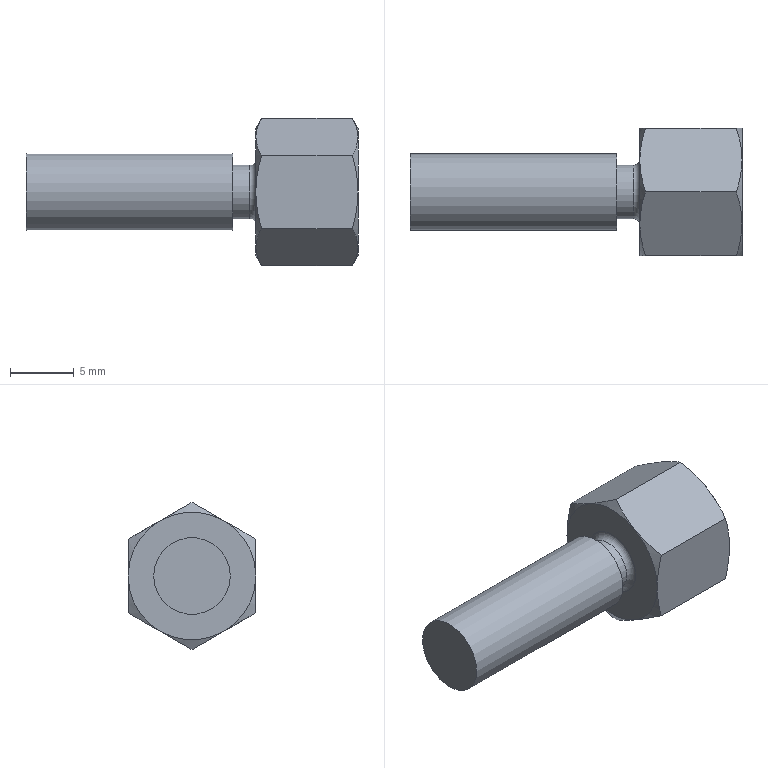Part | NX | features 5003_319_JPRAM6-L8.00-F18 2 | 1 solid | 25 faces | box 26 x 10 x 11.547 mm | volume 1174 mm3 | cone 12 | plane 10 | cylinder 2 | torus 1 | commonest cylinder face diameters 4.2 x1 6 x1
STEP:
#1=CARTESIAN_POINT('',(36.078,-172.,-214.226));
#2=VERTEX_POINT('',#1);
#3=CARTESIAN_POINT('',(28.972,-172.,-214.226));
#4=VERTEX_POINT('',#3);
#5=CARTESIAN_POINT('',(36.525,-172.,-214.226));
#6=DIRECTION('',(-1.,0.,0.));
#7=VECTOR('',#6,1000.);
#8=LINE('',#5,#7);
#9=EDGE_CURVE('',#2,#4,#8,.T.);
#10=ORIENTED_EDGE('',*,*,#9,.F.);
#11=CARTESIAN_POINT('',(36.525,-169.5,-215.67));
#12=VERTEX_POINT('',#11);
#13=CARTESIAN_POINT('',(36.078,-172.,-214.226));
#14=CARTESIAN_POINT('',(36.351,-171.182,-214.699));
#15=CARTESIAN_POINT('',(36.525,-170.352,-215.178));
#16=CARTESIAN_POINT('',(36.525,-169.5,-215.67));
#17=B_SPLINE_CURVE_WITH_KNOTS('',3,(#13,#14,#15,#16),.UNSPECIFIED.,.F.,.F.,(4,4),(0.000000238,0.002921),.UNSPECIFIED.);
#18=EDGE_CURVE('',#2,#12,#17,.T.);
#19=ORIENTED_EDGE('',*,*,#18,.T.);
#20=CARTESIAN_POINT('',(36.078,-167.,-217.113));
#21=VERTEX_POINT('',#20);
#22=CARTESIAN_POINT('',(36.525,-169.5,-215.67));
#23=CARTESIAN_POINT('',(36.525,-168.651,-216.16));
#24=CARTESIAN_POINT('',(36.35,-167.816,-216.642));
#25=CARTESIAN_POINT('',(36.078,-167.,-217.113));
#26=B_SPLINE_CURVE_WITH_KNOTS('',3,(#22,#23,#24,#25),.UNSPECIFIED.,.F.,.F.,(4,4),(0.002921,0.005831),.UNSPECIFIED.);
#27=EDGE_CURVE('',#12,#21,#26,.T.);
#28=ORIENTED_EDGE('',*,*,#27,.T.);
#29=CARTESIAN_POINT('',(28.972,-167.,-217.113));
#30=VERTEX_POINT('',#29);
#31=CARTESIAN_POINT('',(36.525,-167.,-217.113));
#32=DIRECTION('',(-1.,0.,0.));
#33=VECTOR('',#32,1000.);
#34=LINE('',#31,#33);
#35=EDGE_CURVE('',#21,#30,#34,.T.);
#36=ORIENTED_EDGE('',*,*,#35,.T.);
#37=CARTESIAN_POINT('',(28.525,-169.5,-215.67));
#38=VERTEX_POINT('',#37);
#39=CARTESIAN_POINT('',(28.972,-167.,-217.113));
#40=CARTESIAN_POINT('',(28.699,-167.818,-216.641));
#41=CARTESIAN_POINT('',(28.525,-168.648,-216.162));
#42=CARTESIAN_POINT('',(28.525,-169.5,-215.67));
#43=B_SPLINE_CURVE_WITH_KNOTS('',3,(#39,#40,#41,#42),.UNSPECIFIED.,.F.,.F.,(4,4),(0.000000238,0.002921),.UNSPECIFIED.);
#44=EDGE_CURVE('',#30,#38,#43,.T.);
#45=ORIENTED_EDGE('',*,*,#44,.T.);
#46=CARTESIAN_POINT('',(28.525,-169.5,-215.67));
#47=CARTESIAN_POINT('',(28.525,-170.349,-215.18));
#48=CARTESIAN_POINT('',(28.7,-171.184,-214.698));
#49=CARTESIAN_POINT('',(28.972,-172.,-214.226));
#50=B_SPLINE_CURVE_WITH_KNOTS('',3,(#46,#47,#48,#49),.UNSPECIFIED.,.F.,.F.,(4,4),(0.002921,0.005831),.UNSPECIFIED.);
#51=EDGE_CURVE('',#38,#4,#50,.T.);
#52=ORIENTED_EDGE('',*,*,#51,.T.);
#53=EDGE_LOOP('',(#10,#19,#28,#36,#45,#52));
#54=FACE_BOUND('',#53,.T.);
#55=CARTESIAN_POINT('',(36.525,-172.,-214.226));
#56=DIRECTION('',(0.,0.5,0.866));
#57=DIRECTION('',(0.,-0.866,0.5));
#58=AXIS2_PLACEMENT_3D('',#55,#56,#57);
#59=PLANE('',#58);
#60=ADVANCED_FACE('',(#54),#59,.T.);
#61=ORIENTED_EDGE('',*,*,#35,.F.);
#62=CARTESIAN_POINT('',(36.525,-167.,-220.));
#63=VERTEX_POINT('',#62);
#64=CARTESIAN_POINT('',(36.525,-167.,-220.));
#65=CARTESIAN_POINT('',(36.525,-167.,-219.024));
#66=CARTESIAN_POINT('',(36.348,-167.,-218.047));
#67=CARTESIAN_POINT('',(36.078,-167.,-217.113));
#68=B_SPLINE_CURVE_WITH_KNOTS('',3,(#64,#65,#66,#67),.UNSPECIFIED.,.F.,.F.,(4,4),(0.008071,0.01099),.UNSPECIFIED.);
#69=EDGE_CURVE('',#21,#63,#68,.F.);
#70=ORIENTED_EDGE('',*,*,#69,.T.);
#71=CARTESIAN_POINT('',(36.078,-167.,-222.887));
#72=VERTEX_POINT('',#71);
#73=CARTESIAN_POINT('',(36.078,-167.,-222.887));
#74=CARTESIAN_POINT('',(36.349,-167.,-221.948));
#75=CARTESIAN_POINT('',(36.525,-167.,-220.976));
#76=CARTESIAN_POINT('',(36.525,-167.,-220.));
#77=B_SPLINE_CURVE_WITH_KNOTS('',3,(#73,#74,#75,#76),.UNSPECIFIED.,.F.,.F.,(4,4),(0.00515,0.008071),.UNSPECIFIED.);
#78=EDGE_CURVE('',#63,#72,#77,.F.);
#79=ORIENTED_EDGE('',*,*,#78,.T.);
#80=CARTESIAN_POINT('',(28.972,-167.,-222.887));
#81=VERTEX_POINT('',#80);
#82=CARTESIAN_POINT('',(36.525,-167.,-222.887));
#83=DIRECTION('',(-1.,0.,0.));
#84=VECTOR('',#83,1000.);
#85=LINE('',#82,#84);
#86=EDGE_CURVE('',#72,#81,#85,.T.);
#87=ORIENTED_EDGE('',*,*,#86,.T.);
#88=CARTESIAN_POINT('',(28.525,-167.,-220.));
#89=VERTEX_POINT('',#88);
#90=CARTESIAN_POINT('',(28.972,-167.,-222.887));
#91=CARTESIAN_POINT('',(28.701,-167.,-221.948));
#92=CARTESIAN_POINT('',(28.525,-167.,-220.976));
#93=CARTESIAN_POINT('',(28.525,-167.,-220.));
#94=B_SPLINE_CURVE_WITH_KNOTS('',3,(#90,#91,#92,#93),.UNSPECIFIED.,.F.,.F.,(4,4),(0.00515,0.008071),.UNSPECIFIED.);
#95=EDGE_CURVE('',#81,#89,#94,.T.);
#96=ORIENTED_EDGE('',*,*,#95,.T.);
#97=CARTESIAN_POINT('',(28.525,-167.,-220.));
#98=CARTESIAN_POINT('',(28.525,-167.,-219.024));
#99=CARTESIAN_POINT('',(28.702,-167.,-218.047));
#100=CARTESIAN_POINT('',(28.972,-167.,-217.113));
#101=B_SPLINE_CURVE_WITH_KNOTS('',3,(#97,#98,#99,#100),.UNSPECIFIED.,.F.,.F.,(4,4),(0.008071,0.01099),.UNSPECIFIED.);
#102=EDGE_CURVE('',#89,#30,#101,.T.);
#103=ORIENTED_EDGE('',*,*,#102,.T.);
#104=EDGE_LOOP('',(#61,#70,#79,#87,#96,#103));
#105=FACE_BOUND('',#104,.T.);
#106=CARTESIAN_POINT('',(36.525,-167.,-217.113));
#107=DIRECTION('',(0.,1.,0.));
#108=DIRECTION('',(0.,0.,1.));
#109=AXIS2_PLACEMENT_3D('',#106,#107,#108);
#110=PLANE('',#109);
#111=ADVANCED_FACE('',(#105),#110,.T.);
#112=ORIENTED_EDGE('',*,*,#86,.F.);
#113=CARTESIAN_POINT('',(36.525,-169.5,-224.33));
#114=VERTEX_POINT('',#113);
#115=CARTESIAN_POINT('',(36.078,-167.,-222.887));
#116=CARTESIAN_POINT('',(36.351,-167.818,-223.359));
#117=CARTESIAN_POINT('',(36.525,-168.648,-223.838));
#118=CARTESIAN_POINT('',(36.525,-169.5,-224.33));
#119=B_SPLINE_CURVE_WITH_KNOTS('',3,(#115,#116,#117,#118),.UNSPECIFIED.,.F.,.F.,(4,4),(0.000000238,0.002921),.UNSPECIFIED.);
#120=EDGE_CURVE('',#72,#114,#119,.T.);
#121=ORIENTED_EDGE('',*,*,#120,.T.);
#122=CARTESIAN_POINT('',(36.078,-172.,-225.774));
#123=VERTEX_POINT('',#122);
#124=CARTESIAN_POINT('',(36.525,-169.5,-224.33));
#125=CARTESIAN_POINT('',(36.525,-170.349,-224.82));
#126=CARTESIAN_POINT('',(36.35,-171.184,-225.302));
#127=CARTESIAN_POINT('',(36.078,-172.,-225.774));
#128=B_SPLINE_CURVE_WITH_KNOTS('',3,(#124,#125,#126,#127),.UNSPECIFIED.,.F.,.F.,(4,4),(0.002921,0.005831),.UNSPECIFIED.);
#129=EDGE_CURVE('',#114,#123,#128,.T.);
#130=ORIENTED_EDGE('',*,*,#129,.T.);
#131=CARTESIAN_POINT('',(28.972,-172.,-225.774));
#132=VERTEX_POINT('',#131);
#133=CARTESIAN_POINT('',(36.525,-172.,-225.774));
#134=DIRECTION('',(-1.,0.,0.));
#135=VECTOR('',#134,1000.);
#136=LINE('',#133,#135);
#137=EDGE_CURVE('',#123,#132,#136,.T.);
#138=ORIENTED_EDGE('',*,*,#137,.T.);
#139=CARTESIAN_POINT('',(28.525,-169.5,-224.33));
#140=VERTEX_POINT('',#139);
#141=CARTESIAN_POINT('',(28.972,-172.,-225.774));
#142=CARTESIAN_POINT('',(28.699,-171.182,-225.301));
#143=CARTESIAN_POINT('',(28.525,-170.352,-224.822));
#144=CARTESIAN_POINT('',(28.525,-169.5,-224.33));
#145=B_SPLINE_CURVE_WITH_KNOTS('',3,(#141,#142,#143,#144),.UNSPECIFIED.,.F.,.F.,(4,4),(0.000000238,0.002921),.UNSPECIFIED.);
#146=EDGE_CURVE('',#132,#140,#145,.T.);
#147=ORIENTED_EDGE('',*,*,#146,.T.);
#148=CARTESIAN_POINT('',(28.525,-169.5,-224.33));
#149=CARTESIAN_POINT('',(28.525,-168.651,-223.84));
#150=CARTESIAN_POINT('',(28.7,-167.816,-223.358));
#151=CARTESIAN_POINT('',(28.972,-167.,-222.887));
#152=B_SPLINE_CURVE_WITH_KNOTS('',3,(#148,#149,#150,#151),.UNSPECIFIED.,.F.,.F.,(4,4),(0.002921,0.005831),.UNSPECIFIED.);
#153=EDGE_CURVE('',#140,#81,#152,.T.);
#154=ORIENTED_EDGE('',*,*,#153,.T.);
#155=EDGE_LOOP('',(#112,#121,#130,#138,#147,#154));
#156=FACE_BOUND('',#155,.T.);
#157=CARTESIAN_POINT('',(36.525,-167.,-222.887));
#158=DIRECTION('',(0.,0.5,-0.866));
#159=DIRECTION('',(0.,0.866,0.5));
#160=AXIS2_PLACEMENT_3D('',#157,#158,#159);
#161=PLANE('',#160);
#162=ADVANCED_FACE('',(#156),#161,.T.);
#163=ORIENTED_EDGE('',*,*,#137,.F.);
#164=CARTESIAN_POINT('',(36.525,-174.5,-224.33));
#165=VERTEX_POINT('',#164);
#166=CARTESIAN_POINT('',(36.078,-172.,-225.774));
#167=CARTESIAN_POINT('',(36.351,-172.818,-225.301));
#168=CARTESIAN_POINT('',(36.525,-173.648,-224.822));
#169=CARTESIAN_POINT('',(36.525,-174.5,-224.33));
#170=B_SPLINE_CURVE_WITH_KNOTS('',3,(#166,#167,#168,#169),.UNSPECIFIED.,.F.,.F.,(4,4),(0.000000238,0.002921),.UNSPECIFIED.);
#171=EDGE_CURVE('',#123,#165,#170,.T.);
#172=ORIENTED_EDGE('',*,*,#171,.T.);
#173=CARTESIAN_POINT('',(36.078,-177.,-222.887));
#174=VERTEX_POINT('',#173);
#175=CARTESIAN_POINT('',(36.525,-174.5,-224.33));
#176=CARTESIAN_POINT('',(36.525,-175.349,-223.84));
#177=CARTESIAN_POINT('',(36.35,-176.184,-223.358));
#178=CARTESIAN_POINT('',(36.078,-177.,-222.887));
#179=B_SPLINE_CURVE_WITH_KNOTS('',3,(#175,#176,#177,#178),.UNSPECIFIED.,.F.,.F.,(4,4),(0.002921,0.005831),.UNSPECIFIED.);
#180=EDGE_CURVE('',#165,#174,#179,.T.);
#181=ORIENTED_EDGE('',*,*,#180,.T.);
#182=CARTESIAN_POINT('',(28.972,-177.,-222.887));
#183=VERTEX_POINT('',#182);
#184=CARTESIAN_POINT('',(36.525,-177.,-222.887));
#185=DIRECTION('',(-1.,0.,0.));
#186=VECTOR('',#185,1000.);
#187=LINE('',#184,#186);
#188=EDGE_CURVE('',#174,#183,#187,.T.);
#189=ORIENTED_EDGE('',*,*,#188,.T.);
#190=CARTESIAN_POINT('',(28.525,-174.5,-224.33));
#191=VERTEX_POINT('',#190);
#192=CARTESIAN_POINT('',(28.972,-177.,-222.887));
#193=CARTESIAN_POINT('',(28.699,-176.182,-223.359));
#194=CARTESIAN_POINT('',(28.525,-175.352,-223.838));
#195=CARTESIAN_POINT('',(28.525,-174.5,-224.33));
#196=B_SPLINE_CURVE_WITH_KNOTS('',3,(#192,#193,#194,#195),.UNSPECIFIED.,.F.,.F.,(4,4),(0.000000238,0.002921),.UNSPECIFIED.);
#197=EDGE_CURVE('',#183,#191,#196,.T.);
#198=ORIENTED_EDGE('',*,*,#197,.T.);
#199=CARTESIAN_POINT('',(28.525,-174.5,-224.33));
#200=CARTESIAN_POINT('',(28.525,-173.651,-224.82));
#201=CARTESIAN_POINT('',(28.7,-172.816,-225.302));
#202=CARTESIAN_POINT('',(28.972,-172.,-225.774));
#203=B_SPLINE_CURVE_WITH_KNOTS('',3,(#199,#200,#201,#202),.UNSPECIFIED.,.F.,.F.,(4,4),(0.002921,0.005831),.UNSPECIFIED.);
#204=EDGE_CURVE('',#191,#132,#203,.T.);
#205=ORIENTED_EDGE('',*,*,#204,.T.);
#206=EDGE_LOOP('',(#163,#172,#181,#189,#198,#205));
#207=FACE_BOUND('',#206,.T.);
#208=CARTESIAN_POINT('',(36.525,-172.,-225.774));
#209=DIRECTION('',(0.,-0.5,-0.866));
#210=DIRECTION('',(0.,0.866,-0.5));
#211=AXIS2_PLACEMENT_3D('',#208,#209,#210);
#212=PLANE('',#211);
#213=ADVANCED_FACE('',(#207),#212,.T.);
#214=ORIENTED_EDGE('',*,*,#188,.F.);
#215=CARTESIAN_POINT('',(36.525,-177.,-220.));
#216=VERTEX_POINT('',#215);
#217=CARTESIAN_POINT('',(36.078,-177.,-222.887));
#218=CARTESIAN_POINT('',(36.349,-177.,-221.948));
#219=CARTESIAN_POINT('',(36.525,-177.,-220.976));
#220=CARTESIAN_POINT('',(36.525,-177.,-220.));
#221=B_SPLINE_CURVE_WITH_KNOTS('',3,(#217,#218,#219,#220),.UNSPECIFIED.,.F.,.F.,(4,4),(0.00515,0.008071),.UNSPECIFIED.);
#222=EDGE_CURVE('',#174,#216,#221,.T.);
#223=ORIENTED_EDGE('',*,*,#222,.T.);
#224=CARTESIAN_POINT('',(36.078,-177.,-217.113));
#225=VERTEX_POINT('',#224);
#226=CARTESIAN_POINT('',(36.525,-177.,-220.));
#227=CARTESIAN_POINT('',(36.525,-177.,-219.024));
#228=CARTESIAN_POINT('',(36.348,-177.,-218.047));
#229=CARTESIAN_POINT('',(36.078,-177.,-217.113));
#230=B_SPLINE_CURVE_WITH_KNOTS('',3,(#226,#227,#228,#229),.UNSPECIFIED.,.F.,.F.,(4,4),(0.008071,0.01099),.UNSPECIFIED.);
#231=EDGE_CURVE('',#216,#225,#230,.T.);
#232=ORIENTED_EDGE('',*,*,#231,.T.);
#233=CARTESIAN_POINT('',(28.972,-177.,-217.113));
#234=VERTEX_POINT('',#233);
#235=CARTESIAN_POINT('',(36.525,-177.,-217.113));
#236=DIRECTION('',(-1.,0.,0.));
#237=VECTOR('',#236,1000.);
#238=LINE('',#235,#237);
#239=EDGE_CURVE('',#225,#234,#238,.T.);
#240=ORIENTED_EDGE('',*,*,#239,.T.);
#241=CARTESIAN_POINT('',(28.525,-177.,-220.));
#242=VERTEX_POINT('',#241);
#243=CARTESIAN_POINT('',(28.525,-177.,-220.));
#244=CARTESIAN_POINT('',(28.525,-177.,-219.024));
#245=CARTESIAN_POINT('',(28.702,-177.,-218.047));
#246=CARTESIAN_POINT('',(28.972,-177.,-217.113));
#247=B_SPLINE_CURVE_WITH_KNOTS('',3,(#243,#244,#245,#246),.UNSPECIFIED.,.F.,.F.,(4,4),(0.008071,0.01099),.UNSPECIFIED.);
#248=EDGE_CURVE('',#234,#242,#247,.F.);
#249=ORIENTED_EDGE('',*,*,#248,.T.);
#250=CARTESIAN_POINT('',(28.972,-177.,-222.887));
#251=CARTESIAN_POINT('',(28.701,-177.,-221.948));
#252=CARTESIAN_POINT('',(28.525,-177.,-220.976));
#253=CARTESIAN_POINT('',(28.525,-177.,-220.));
#254=B_SPLINE_CURVE_WITH_KNOTS('',3,(#250,#251,#252,#253),.UNSPECIFIED.,.F.,.F.,(4,4),(0.00515,0.008071),.UNSPECIFIED.);
#255=EDGE_CURVE('',#242,#183,#254,.F.);
#256=ORIENTED_EDGE('',*,*,#255,.T.);
#257=EDGE_LOOP('',(#214,#223,#232,#240,#249,#256));
#258=FACE_BOUND('',#257,.T.);
#259=CARTESIAN_POINT('',(36.525,-177.,-222.887));
#260=DIRECTION('',(0.,-1.,0.));
#261=DIRECTION('',(1.,0.,0.));
#262=AXIS2_PLACEMENT_3D('',#259,#260,#261);
#263=PLANE('',#262);
#264=ADVANCED_FACE('',(#258),#263,.T.);
#265=ORIENTED_EDGE('',*,*,#239,.F.);
#266=CARTESIAN_POINT('',(36.525,-174.5,-215.67));
#267=VERTEX_POINT('',#266);
#268=CARTESIAN_POINT('',(36.078,-177.,-217.113));
#269=CARTESIAN_POINT('',(36.351,-176.182,-216.641));
#270=CARTESIAN_POINT('',(36.525,-175.352,-216.162));
#271=CARTESIAN_POINT('',(36.525,-174.5,-215.67));
#272=B_SPLINE_CURVE_WITH_KNOTS('',3,(#268,#269,#270,#271),.UNSPECIFIED.,.F.,.F.,(4,4),(0.000000238,0.002921),.UNSPECIFIED.);
#273=EDGE_CURVE('',#225,#267,#272,.T.);
#274=ORIENTED_EDGE('',*,*,#273,.T.);
#275=CARTESIAN_POINT('',(36.525,-174.5,-215.67));
#276=CARTESIAN_POINT('',(36.525,-173.651,-215.18));
#277=CARTESIAN_POINT('',(36.35,-172.816,-214.698));
#278=CARTESIAN_POINT('',(36.078,-172.,-214.226));
#279=B_SPLINE_CURVE_WITH_KNOTS('',3,(#275,#276,#277,#278),.UNSPECIFIED.,.F.,.F.,(4,4),(0.002921,0.005831),.UNSPECIFIED.);
#280=EDGE_CURVE('',#267,#2,#279,.T.);
#281=ORIENTED_EDGE('',*,*,#280,.T.);
#282=ORIENTED_EDGE('',*,*,#9,.T.);
#283=CARTESIAN_POINT('',(28.525,-174.5,-215.67));
#284=VERTEX_POINT('',#283);
#285=CARTESIAN_POINT('',(28.972,-172.,-214.226));
#286=CARTESIAN_POINT('',(28.699,-172.818,-214.699));
#287=CARTESIAN_POINT('',(28.525,-173.648,-215.178));
#288=CARTESIAN_POINT('',(28.525,-174.5,-215.67));
#289=B_SPLINE_CURVE_WITH_KNOTS('',3,(#285,#286,#287,#288),.UNSPECIFIED.,.F.,.F.,(4,4),(0.000000238,0.002921),.UNSPECIFIED.);
#290=EDGE_CURVE('',#4,#284,#289,.T.);
#291=ORIENTED_EDGE('',*,*,#290,.T.);
#292=CARTESIAN_POINT('',(28.525,-174.5,-215.67));
#293=CARTESIAN_POINT('',(28.525,-175.349,-216.16));
#294=CARTESIAN_POINT('',(28.7,-176.184,-216.642));
#295=CARTESIAN_POINT('',(28.972,-177.,-217.113));
#296=B_SPLINE_CURVE_WITH_KNOTS('',3,(#292,#293,#294,#295),.UNSPECIFIED.,.F.,.F.,(4,4),(0.002921,0.005831),.UNSPECIFIED.);
#297=EDGE_CURVE('',#284,#234,#296,.T.);
#298=ORIENTED_EDGE('',*,*,#297,.T.);
#299=EDGE_LOOP('',(#265,#274,#281,#282,#291,#298));
#300=FACE_BOUND('',#299,.T.);
#301=CARTESIAN_POINT('',(36.525,-177.,-217.113));
#302=DIRECTION('',(0.,-0.5,0.866));
#303=DIRECTION('',(0.,-0.866,-0.5));
#304=AXIS2_PLACEMENT_3D('',#301,#302,#303);
#305=PLANE('',#304);
#306=ADVANCED_FACE('',(#300),#305,.T.);
#307=CARTESIAN_POINT('',(28.525,-169.4,-220.));
#308=VERTEX_POINT('',#307);
#309=CARTESIAN_POINT('',(28.525,-172.,-220.));
#310=DIRECTION('',(1.,0.,0.));
#311=DIRECTION('',(0.,1.,0.));
#312=AXIS2_PLACEMENT_3D('',#309,#310,#311);
#313=CIRCLE('',#312,2.6);
#314=EDGE_CURVE('',#308,#308,#313,.T.);
#315=ORIENTED_EDGE('',*,*,#314,.T.);
#316=EDGE_LOOP('',(#315));
#317=FACE_BOUND('',#316,.T.);
#318=CARTESIAN_POINT('',(28.525,-172.,-220.));
#319=DIRECTION('',(-1.,0.,0.));
#320=DIRECTION('',(0.,-1.,0.));
#321=AXIS2_PLACEMENT_3D('',#318,#319,#320);
#322=CIRCLE('',#321,5.);
#323=EDGE_CURVE('',#38,#89,#322,.T.);
#324=ORIENTED_EDGE('',*,*,#323,.T.);
#325=CARTESIAN_POINT('',(28.525,-172.,-220.));
#326=DIRECTION('',(-1.,0.,0.));
#327=DIRECTION('',(0.,-1.,0.));
#328=AXIS2_PLACEMENT_3D('',#325,#326,#327);
#329=CIRCLE('',#328,5.);
#330=EDGE_CURVE('',#89,#140,#329,.T.);
#331=ORIENTED_EDGE('',*,*,#330,.T.);
#332=CARTESIAN_POINT('',(28.525,-172.,-220.));
#333=DIRECTION('',(-1.,0.,0.));
#334=DIRECTION('',(0.,-1.,0.));
#335=AXIS2_PLACEMENT_3D('',#332,#333,#334);
#336=CIRCLE('',#335,5.);
#337=EDGE_CURVE('',#140,#191,#336,.T.);
#338=ORIENTED_EDGE('',*,*,#337,.T.);
#339=CARTESIAN_POINT('',(28.525,-172.,-220.));
#340=DIRECTION('',(-1.,0.,0.));
#341=DIRECTION('',(0.,-1.,0.));
#342=AXIS2_PLACEMENT_3D('',#339,#340,#341);
#343=CIRCLE('',#342,5.);
#344=EDGE_CURVE('',#191,#242,#343,.T.);
#345=ORIENTED_EDGE('',*,*,#344,.T.);
#346=CARTESIAN_POINT('',(28.525,-172.,-220.));
#347=DIRECTION('',(-1.,0.,0.));
#348=DIRECTION('',(0.,-1.,0.));
#349=AXIS2_PLACEMENT_3D('',#346,#347,#348);
#350=CIRCLE('',#349,5.);
#351=EDGE_CURVE('',#242,#284,#350,.T.);
#352=ORIENTED_EDGE('',*,*,#351,.T.);
#353=CARTESIAN_POINT('',(28.525,-172.,-220.));
#354=DIRECTION('',(-1.,0.,0.));
#355=DIRECTION('',(0.,-1.,0.));
#356=AXIS2_PLACEMENT_3D('',#353,#354,#355);
#357=CIRCLE('',#356,5.);
#358=EDGE_CURVE('',#284,#38,#357,.T.);
#359=ORIENTED_EDGE('',*,*,#358,.T.);
#360=EDGE_LOOP('',(#324,#331,#338,#345,#352,#359));
#361=FACE_BOUND('',#360,.T.);
#362=CARTESIAN_POINT('',(28.525,-172.,-217.9));
#363=DIRECTION('',(1.,0.,0.));
#364=DIRECTION('',(0.,1.,0.));
#365=AXIS2_PLACEMENT_3D('',#362,#363,#364);
#366=PLANE('',#365);
#367=ADVANCED_FACE('',(#317,#361),#366,.F.);
#368=CARTESIAN_POINT('',(10.525,-175.,-220.));
#369=VERTEX_POINT('',#368);
#370=CARTESIAN_POINT('',(10.525,-172.,-220.));
#371=DIRECTION('',(-1.,0.,0.));
#372=DIRECTION('',(0.,-1.,0.));
#373=AXIS2_PLACEMENT_3D('',#370,#371,#372);
#374=CIRCLE('',#373,3.);
#375=EDGE_CURVE('',#369,#369,#374,.T.);
#376=ORIENTED_EDGE('',*,*,#375,.T.);
#377=EDGE_LOOP('',(#376));
#378=FACE_BOUND('',#377,.T.);
#379=CARTESIAN_POINT('',(10.525,-172.,-220.));
#380=DIRECTION('',(1.,0.,0.));
#381=DIRECTION('',(0.,1.,0.));
#382=AXIS2_PLACEMENT_3D('',#379,#380,#381);
#383=PLANE('',#382);
#384=ADVANCED_FACE('',(#378),#383,.F.);
#385=ORIENTED_EDGE('',*,*,#375,.F.);
#386=EDGE_LOOP('',(#385));
#387=FACE_BOUND('',#386,.T.);
#388=CARTESIAN_POINT('',(26.725,-175.,-220.));
#389=VERTEX_POINT('',#388);
#390=CARTESIAN_POINT('',(26.725,-172.,-220.));
#391=DIRECTION('',(-1.,0.,0.));
#392=DIRECTION('',(0.,-1.,0.));
#393=AXIS2_PLACEMENT_3D('',#390,#391,#392);
#394=CIRCLE('',#393,3.);
#395=EDGE_CURVE('',#389,#389,#394,.T.);
#396=ORIENTED_EDGE('',*,*,#395,.T.);
#397=EDGE_LOOP('',(#396));
#398=FACE_BOUND('',#397,.T.);
#399=CARTESIAN_POINT('',(10.525,-172.,-220.));
#400=DIRECTION('',(-1.,0.,0.));
#401=DIRECTION('',(0.,-1.,0.));
#402=AXIS2_PLACEMENT_3D('',#399,#400,#401);
#403=CYLINDRICAL_SURFACE('',#402,3.);
#404=ADVANCED_FACE('',(#387,#398),#403,.T.);
#405=ORIENTED_EDGE('',*,*,#395,.F.);
#406=EDGE_LOOP('',(#405));
#407=FACE_BOUND('',#406,.T.);
#408=CARTESIAN_POINT('',(26.725,-174.1,-220.));
#409=VERTEX_POINT('',#408);
#410=CARTESIAN_POINT('',(26.725,-172.,-220.));
#411=DIRECTION('',(-1.,0.,0.));
#412=DIRECTION('',(0.,-1.,0.));
#413=AXIS2_PLACEMENT_3D('',#410,#411,#412);
#414=CIRCLE('',#413,2.1);
#415=EDGE_CURVE('',#409,#409,#414,.T.);
#416=ORIENTED_EDGE('',*,*,#415,.T.);
#417=EDGE_LOOP('',(#416));
#418=FACE_BOUND('',#417,.T.);
#419=CARTESIAN_POINT('',(26.725,-172.,-217.));
#420=DIRECTION('',(-1.,0.,0.));
#421=DIRECTION('',(0.,-1.,0.));
#422=AXIS2_PLACEMENT_3D('',#419,#420,#421);
#423=PLANE('',#422);
#424=ADVANCED_FACE('',(#407,#418),#423,.F.);
#425=CARTESIAN_POINT('',(28.025,-169.9,-220.));
#426=VERTEX_POINT('',#425);
#427=CARTESIAN_POINT('',(28.025,-172.,-220.));
#428=DIRECTION('',(1.,0.,0.));
#429=DIRECTION('',(0.,1.,0.));
#430=AXIS2_PLACEMENT_3D('',#427,#428,#429);
#431=CIRCLE('',#430,2.1);
#432=EDGE_CURVE('',#426,#426,#431,.F.);
#433=ORIENTED_EDGE('',*,*,#432,.T.);
#434=EDGE_LOOP('',(#433));
#435=FACE_BOUND('',#434,.T.);
#436=ORIENTED_EDGE('',*,*,#415,.F.);
#437=EDGE_LOOP('',(#436));
#438=FACE_BOUND('',#437,.T.);
#439=CARTESIAN_POINT('',(10.525,-172.,-220.));
#440=DIRECTION('',(-1.,0.,0.));
#441=DIRECTION('',(0.,-1.,0.));
#442=AXIS2_PLACEMENT_3D('',#439,#440,#441);
#443=CYLINDRICAL_SURFACE('',#442,2.1);
#444=ADVANCED_FACE('',(#435,#438),#443,.T.);
#445=ORIENTED_EDGE('',*,*,#51,.F.);
#446=ORIENTED_EDGE('',*,*,#358,.F.);
#447=ORIENTED_EDGE('',*,*,#290,.F.);
#448=EDGE_LOOP('',(#445,#446,#447));
#449=FACE_BOUND('',#448,.T.);
#450=CARTESIAN_POINT('',(28.525,-172.,-220.));
#451=DIRECTION('',(1.,0.,0.));
#452=DIRECTION('',(0.,1.,0.));
#453=AXIS2_PLACEMENT_3D('',#450,#451,#452);
#454=CONICAL_SURFACE('',#453,5.,1.047);
#455=ADVANCED_FACE('',(#449),#454,.T.);
#456=ORIENTED_EDGE('',*,*,#323,.F.);
#457=ORIENTED_EDGE('',*,*,#44,.F.);
#458=ORIENTED_EDGE('',*,*,#102,.F.);
#459=EDGE_LOOP('',(#456,#457,#458));
#460=FACE_BOUND('',#459,.T.);
#461=CARTESIAN_POINT('',(28.525,-172.,-220.));
#462=DIRECTION('',(1.,0.,0.));
#463=DIRECTION('',(0.,1.,0.));
#464=AXIS2_PLACEMENT_3D('',#461,#462,#463);
#465=CONICAL_SURFACE('',#464,5.,1.047);
#466=ADVANCED_FACE('',(#460),#465,.T.);
#467=ORIENTED_EDGE('',*,*,#330,.F.);
#468=ORIENTED_EDGE('',*,*,#95,.F.);
#469=ORIENTED_EDGE('',*,*,#153,.F.);
#470=EDGE_LOOP('',(#467,#468,#469));
#471=FACE_BOUND('',#470,.T.);
#472=CARTESIAN_POINT('',(28.525,-172.,-220.));
#473=DIRECTION('',(1.,0.,0.));
#474=DIRECTION('',(0.,1.,0.));
#475=AXIS2_PLACEMENT_3D('',#472,#473,#474);
#476=CONICAL_SURFACE('',#475,5.,1.047);
#477=ADVANCED_FACE('',(#471),#476,.T.);
#478=ORIENTED_EDGE('',*,*,#337,.F.);
#479=ORIENTED_EDGE('',*,*,#146,.F.);
#480=ORIENTED_EDGE('',*,*,#204,.F.);
#481=EDGE_LOOP('',(#478,#479,#480));
#482=FACE_BOUND('',#481,.T.);
#483=CARTESIAN_POINT('',(28.525,-172.,-220.));
#484=DIRECTION('',(1.,0.,0.));
#485=DIRECTION('',(0.,1.,0.));
#486=AXIS2_PLACEMENT_3D('',#483,#484,#485);
#487=CONICAL_SURFACE('',#486,5.,1.047);
#488=ADVANCED_FACE('',(#482),#487,.T.);
#489=ORIENTED_EDGE('',*,*,#344,.F.);
#490=ORIENTED_EDGE('',*,*,#197,.F.);
#491=ORIENTED_EDGE('',*,*,#255,.F.);
#492=EDGE_LOOP('',(#489,#490,#491));
#493=FACE_BOUND('',#492,.T.);
#494=CARTESIAN_POINT('',(28.525,-172.,-220.));
#495=DIRECTION('',(1.,0.,0.));
#496=DIRECTION('',(0.,1.,0.));
#497=AXIS2_PLACEMENT_3D('',#494,#495,#496);
#498=CONICAL_SURFACE('',#497,5.,1.047);
#499=ADVANCED_FACE('',(#493),#498,.T.);
#500=ORIENTED_EDGE('',*,*,#351,.F.);
#501=ORIENTED_EDGE('',*,*,#248,.F.);
#502=ORIENTED_EDGE('',*,*,#297,.F.);
#503=EDGE_LOOP('',(#500,#501,#502));
#504=FACE_BOUND('',#503,.T.);
#505=CARTESIAN_POINT('',(28.525,-172.,-220.));
#506=DIRECTION('',(1.,0.,0.));
#507=DIRECTION('',(0.,1.,0.));
#508=AXIS2_PLACEMENT_3D('',#505,#506,#507);
#509=CONICAL_SURFACE('',#508,5.,1.047);
#510=ADVANCED_FACE('',(#504),#509,.T.);
#511=ORIENTED_EDGE('',*,*,#280,.F.);
#512=CARTESIAN_POINT('',(36.525,-172.,-220.));
#513=DIRECTION('',(-1.,0.,0.));
#514=DIRECTION('',(0.,-1.,0.));
#515=AXIS2_PLACEMENT_3D('',#512,#513,#514);
#516=CIRCLE('',#515,5.);
#517=EDGE_CURVE('',#267,#12,#516,.T.);
#518=ORIENTED_EDGE('',*,*,#517,.T.);
#519=ORIENTED_EDGE('',*,*,#18,.F.);
#520=EDGE_LOOP('',(#511,#518,#519));
#521=FACE_BOUND('',#520,.T.);
#522=CARTESIAN_POINT('',(36.078,-172.,-220.));
#523=DIRECTION('',(-1.,0.,0.));
#524=DIRECTION('',(0.,-1.,0.));
#525=AXIS2_PLACEMENT_3D('',#522,#523,#524);
#526=CONICAL_SURFACE('',#525,5.774,1.047);
#527=ADVANCED_FACE('',(#521),#526,.T.);
#528=CARTESIAN_POINT('',(36.525,-172.,-220.));
#529=DIRECTION('',(-1.,0.,0.));
#530=DIRECTION('',(0.,-1.,0.));
#531=AXIS2_PLACEMENT_3D('',#528,#529,#530);
#532=CIRCLE('',#531,5.);
#533=EDGE_CURVE('',#216,#267,#532,.T.);
#534=ORIENTED_EDGE('',*,*,#533,.T.);
#535=ORIENTED_EDGE('',*,*,#273,.F.);
#536=ORIENTED_EDGE('',*,*,#231,.F.);
#537=EDGE_LOOP('',(#534,#535,#536));
#538=FACE_BOUND('',#537,.T.);
#539=CARTESIAN_POINT('',(36.078,-172.,-220.));
#540=DIRECTION('',(-1.,0.,0.));
#541=DIRECTION('',(0.,-1.,0.));
#542=AXIS2_PLACEMENT_3D('',#539,#540,#541);
#543=CONICAL_SURFACE('',#542,5.774,1.047);
#544=ADVANCED_FACE('',(#538),#543,.T.);
#545=CARTESIAN_POINT('',(36.525,-172.,-220.));
#546=DIRECTION('',(-1.,0.,0.));
#547=DIRECTION('',(0.,-1.,0.));
#548=AXIS2_PLACEMENT_3D('',#545,#546,#547);
#549=CIRCLE('',#548,5.);
#550=EDGE_CURVE('',#165,#216,#549,.T.);
#551=ORIENTED_EDGE('',*,*,#550,.T.);
#552=ORIENTED_EDGE('',*,*,#222,.F.);
#553=ORIENTED_EDGE('',*,*,#180,.F.);
#554=EDGE_LOOP('',(#551,#552,#553));
#555=FACE_BOUND('',#554,.T.);
#556=CARTESIAN_POINT('',(36.078,-172.,-220.));
#557=DIRECTION('',(-1.,0.,0.));
#558=DIRECTION('',(0.,-1.,0.));
#559=AXIS2_PLACEMENT_3D('',#556,#557,#558);
#560=CONICAL_SURFACE('',#559,5.774,1.047);
#561=ADVANCED_FACE('',(#555),#560,.T.);
#562=CARTESIAN_POINT('',(36.525,-172.,-220.));
#563=DIRECTION('',(-1.,0.,0.));
#564=DIRECTION('',(0.,-1.,0.));
#565=AXIS2_PLACEMENT_3D('',#562,#563,#564);
#566=CIRCLE('',#565,5.);
#567=EDGE_CURVE('',#114,#165,#566,.T.);
#568=ORIENTED_EDGE('',*,*,#567,.T.);
#569=ORIENTED_EDGE('',*,*,#171,.F.);
#570=ORIENTED_EDGE('',*,*,#129,.F.);
#571=EDGE_LOOP('',(#568,#569,#570));
#572=FACE_BOUND('',#571,.T.);
#573=CARTESIAN_POINT('',(36.078,-172.,-220.));
#574=DIRECTION('',(-1.,0.,0.));
#575=DIRECTION('',(0.,-1.,0.));
#576=AXIS2_PLACEMENT_3D('',#573,#574,#575);
#577=CONICAL_SURFACE('',#576,5.774,1.047);
#578=ADVANCED_FACE('',(#572),#577,.T.);
#579=CARTESIAN_POINT('',(36.525,-172.,-220.));
#580=DIRECTION('',(-1.,0.,0.));
#581=DIRECTION('',(0.,-1.,0.));
#582=AXIS2_PLACEMENT_3D('',#579,#580,#581);
#583=CIRCLE('',#582,5.);
#584=EDGE_CURVE('',#63,#114,#583,.T.);
#585=ORIENTED_EDGE('',*,*,#584,.T.);
#586=ORIENTED_EDGE('',*,*,#120,.F.);
#587=ORIENTED_EDGE('',*,*,#78,.F.);
#588=EDGE_LOOP('',(#585,#586,#587));
#589=FACE_BOUND('',#588,.T.);
#590=CARTESIAN_POINT('',(36.078,-172.,-220.));
#591=DIRECTION('',(-1.,0.,0.));
#592=DIRECTION('',(0.,-1.,0.));
#593=AXIS2_PLACEMENT_3D('',#590,#591,#592);
#594=CONICAL_SURFACE('',#593,5.774,1.047);
#595=ADVANCED_FACE('',(#589),#594,.T.);
#596=CARTESIAN_POINT('',(36.525,-172.,-220.));
#597=DIRECTION('',(-1.,0.,0.));
#598=DIRECTION('',(0.,-1.,0.));
#599=AXIS2_PLACEMENT_3D('',#596,#597,#598);
#600=CIRCLE('',#599,5.);
#601=EDGE_CURVE('',#12,#63,#600,.T.);
#602=ORIENTED_EDGE('',*,*,#601,.T.);
#603=ORIENTED_EDGE('',*,*,#69,.F.);
#604=ORIENTED_EDGE('',*,*,#27,.F.);
#605=EDGE_LOOP('',(#602,#603,#604));
#606=FACE_BOUND('',#605,.T.);
#607=CARTESIAN_POINT('',(36.078,-172.,-220.));
#608=DIRECTION('',(-1.,0.,0.));
#609=DIRECTION('',(0.,-1.,0.));
#610=AXIS2_PLACEMENT_3D('',#607,#608,#609);
#611=CONICAL_SURFACE('',#610,5.774,1.047);
#612=ADVANCED_FACE('',(#606),#611,.T.);
#613=ORIENTED_EDGE('',*,*,#533,.F.);
#614=ORIENTED_EDGE('',*,*,#550,.F.);
#615=ORIENTED_EDGE('',*,*,#567,.F.);
#616=ORIENTED_EDGE('',*,*,#584,.F.);
#617=ORIENTED_EDGE('',*,*,#601,.F.);
#618=ORIENTED_EDGE('',*,*,#517,.F.);
#619=EDGE_LOOP('',(#613,#614,#615,#616,#617,#618));
#620=FACE_BOUND('',#619,.T.);
#621=CARTESIAN_POINT('',(36.525,-172.,-217.));
#622=DIRECTION('',(-1.,0.,0.));
#623=DIRECTION('',(0.,-1.,0.));
#624=AXIS2_PLACEMENT_3D('',#621,#622,#623);
#625=PLANE('',#624);
#626=ADVANCED_FACE('',(#620),#625,.F.);
#627=ORIENTED_EDGE('',*,*,#314,.F.);
#628=EDGE_LOOP('',(#627));
#629=FACE_BOUND('',#628,.T.);
#630=ORIENTED_EDGE('',*,*,#432,.F.);
#631=EDGE_LOOP('',(#630));
#632=FACE_BOUND('',#631,.T.);
#633=CARTESIAN_POINT('',(28.025,-172.,-220.));
#634=DIRECTION('',(1.,0.,0.));
#635=DIRECTION('',(0.,1.,0.));
#636=AXIS2_PLACEMENT_3D('',#633,#634,#635);
#637=TOROIDAL_SURFACE('',#636,2.6,0.5);
#638=ADVANCED_FACE('',(#629,#632),#637,.F.);
#639=CLOSED_SHELL('',(#60,#111,#162,#213,#264,#306,#367,#384,#404,#424,#444,#455,#466,#477,#488,#499,#510,#527,#544,#561,#578,#595,#612,#626,#638));
#640=MANIFOLD_SOLID_BREP('',#639);
#641=(LENGTH_UNIT()NAMED_UNIT(*)SI_UNIT(.MILLI.,.METRE.));
#642=UNCERTAINTY_MEASURE_WITH_UNIT(LENGTH_MEASURE(0.0508),#641,'','');
#643=(NAMED_UNIT(*)PLANE_ANGLE_UNIT()SI_UNIT($,.RADIAN.));
#644=(NAMED_UNIT(*)SI_UNIT($,.STERADIAN.)SOLID_ANGLE_UNIT());
#645=(GEOMETRIC_REPRESENTATION_CONTEXT(3)GLOBAL_UNCERTAINTY_ASSIGNED_CONTEXT((#642))GLOBAL_UNIT_ASSIGNED_CONTEXT((#641,#643,#644))REPRESENTATION_CONTEXT('',''));
#646=ADVANCED_BREP_SHAPE_REPRESENTATION('',(#640),#645);